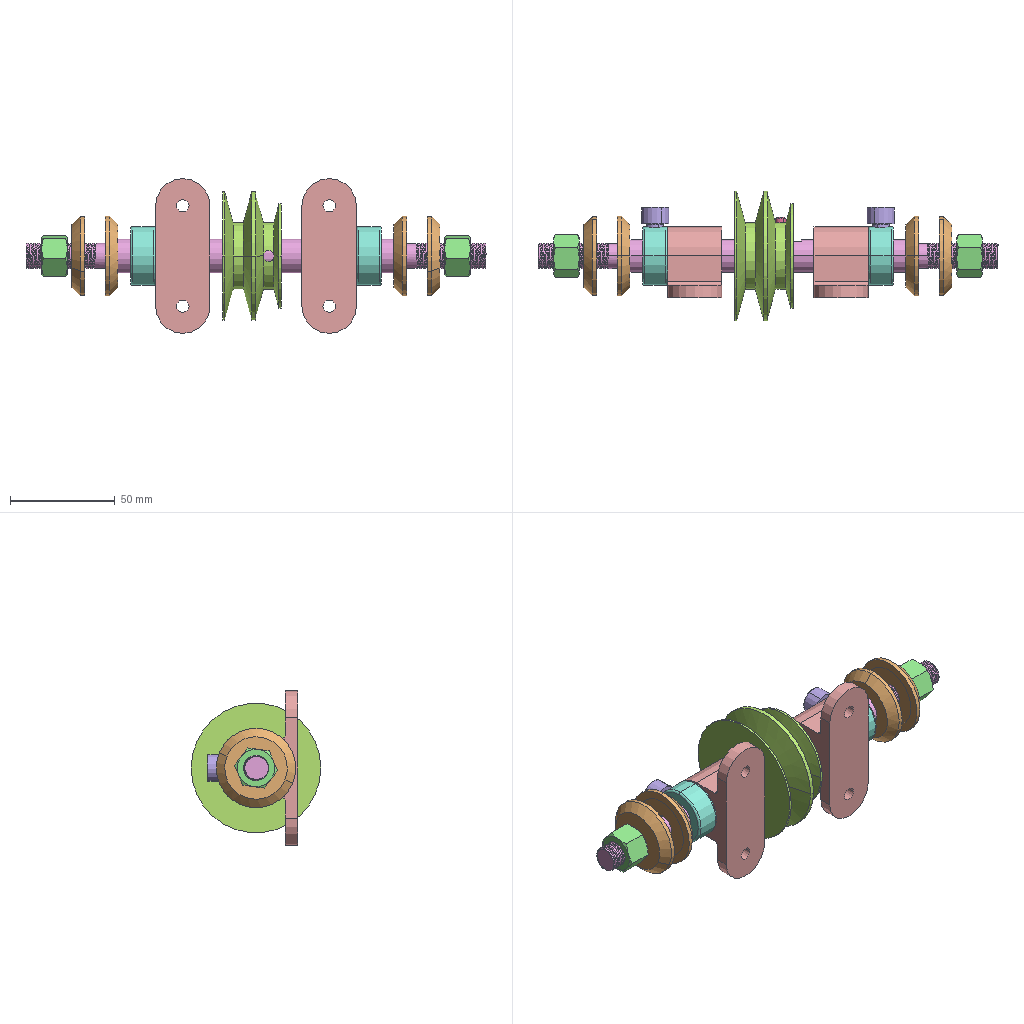Assembly | SolidWorks | 9 different items | 15 placed | box 220 x 62 x 74 mm
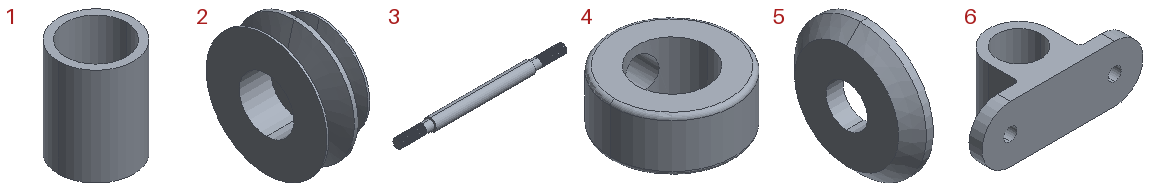Parts list (item | name | quantity | size | volume | features):
1 | - | x2 | 20 x 20 x 26 mm | 2941 mm3 | features Extrusion 1
2 | - | x1 | 28 x 62 x 62 mm | 29856 mm3 | features ICE 2, 3DProfileFeature 1, HoleWzd 1, Revolution 1
3 | - | x1 | 221 x 16 x 16 mm | 35769 mm3 | features Helix 1, ICE 1, MirrorPattern 1, Revolution 1, SweepCut 1
4 | - | x2 | 28 x 28 x 12 mm | 4632 mm3 | features Extrusion 1, Fillet 1, ICE 1
5 | - | x4 | 6 x 38 x 38 mm | 4644 mm3 | features Revolution 1
6 | - | x2 | 74 x 34 x 26 mm | 20408 mm3 | features Extrusion 1, Fillet 1, ICE 1
7 | hex nut gradec_iso | x1 | - | - | -
8 | socket head cap screw_iso | x1 | - | - | -
9 | socket set screw cup point_iso | x1 | - | - | -
Mates (type | each side: item.copy, entity, surface, feature):
Coincident | 3.1 plane | assembly plane | 3 times
Coincident | 2.1 edge | assembly plane
Concentric | 6.1 face cylinder Boss-Extrude2 | 3.1 face cylinder Revolve1
Parallel | 6.1 face plane Boss-Extrude1 | assembly plane
DistanceDim | 2.1 face plane Revolve1 | 6.1 face plane Boss-Extrude1
Concentric | 1.1 face cylinder Boss-Extrude1 | 3.1 face cylinder Revolve1
Coincident | 6.1 face plane Boss-Extrude1 | 1.1 face plane Boss-Extrude1
Concentric | 3.1 face cylinder Revolve1 | 5.1 face cylinder Revolve2
Coincident | 3.1 face plane Revolve1 | 5.1 face plane Revolve2
Concentric | 3.1 face cylinder Revolve1 | 5.2 face cylinder Revolve2
DistanceDim | 5.1 face plane Revolve2 | 5.2 face plane Revolve2
Concentric | 3.1 face cylinder Revolve1 | 4.1 face cylinder Boss-Extrude1
Coincident | 6.1 face plane Boss-Extrude1 | 4.1 face plane Boss-Extrude1
Coincident | 4.1 plane | assembly plane
Concentric | 4.1 face cylinder Cut-Extrude1 | assembly face
Concentric | 2.1 face cylinder Boss-Extrude1 | 3.1 face cylinder Revolve1
Coincident | 2.1 plane | assembly plane